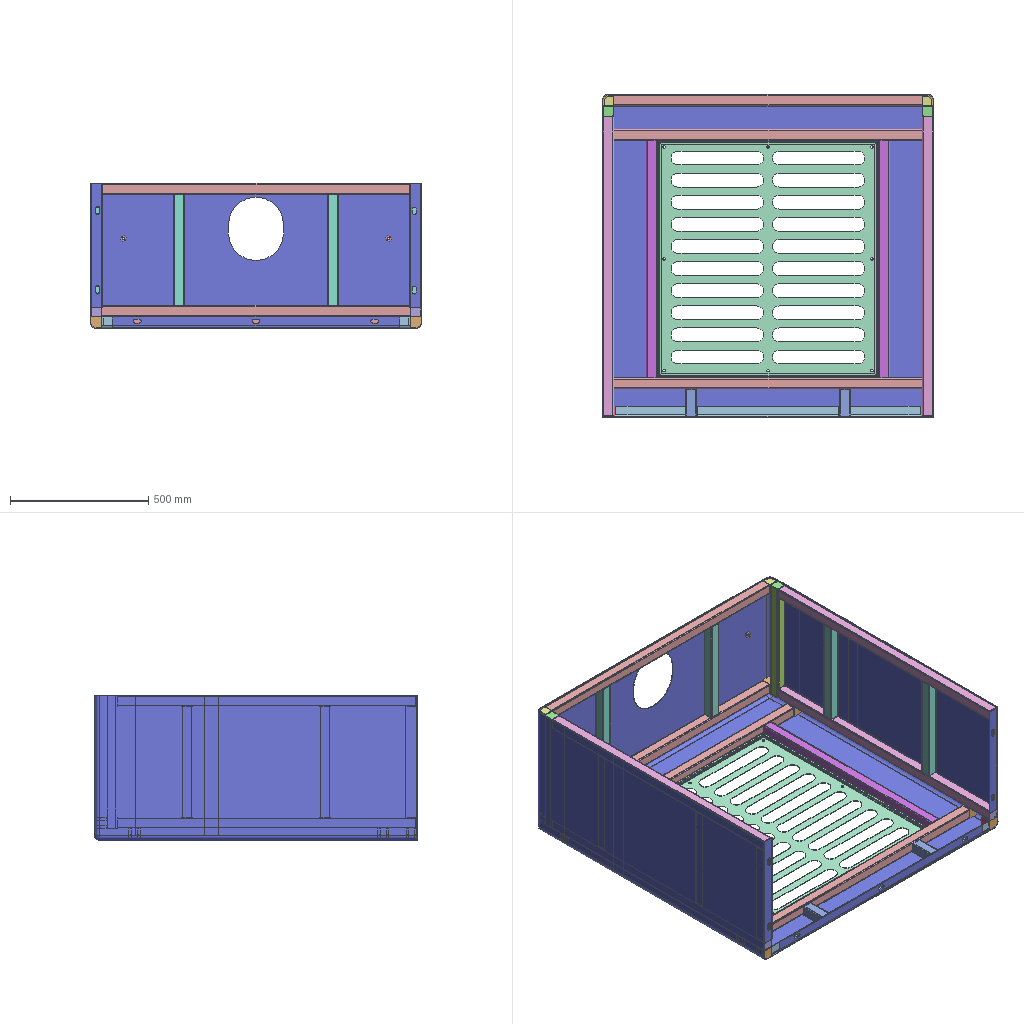Assembly | SolidWorks | 17 different items | 54 placed | box 1200 x 1170 x 527 mm
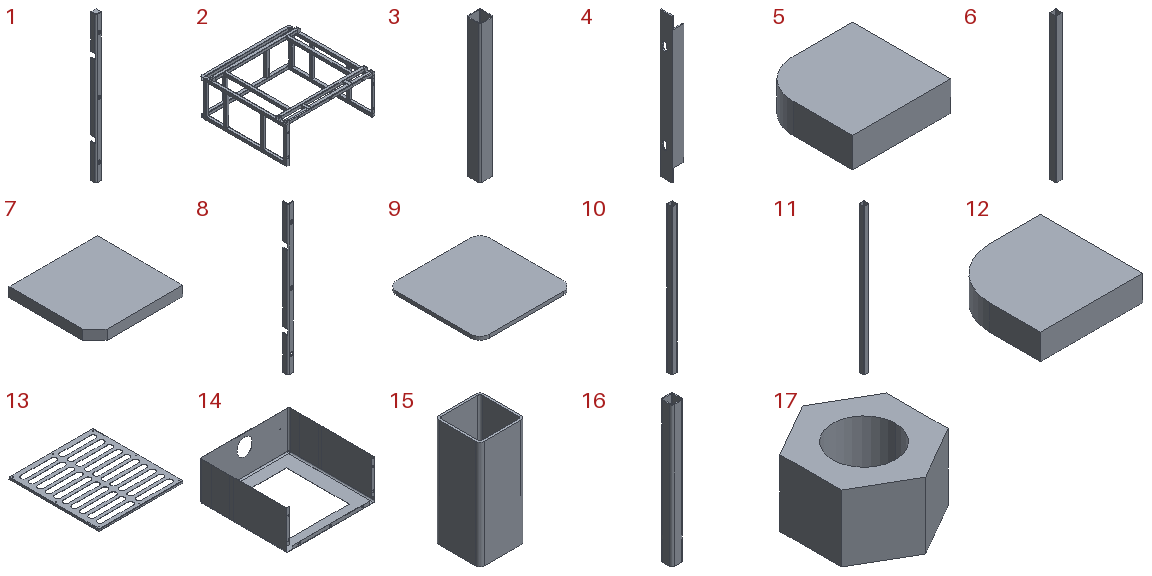Parts list (item | name | quantity | parent item | size | volume | features):
1 | (subassembly) | x1 | in 2 | 40 x 40 x 1116 mm | 321281 mm3 | -
2 | (subassembly) | x1 | - | 1196 x 1166 x 524.14 mm | 5123643 mm3 | features ReferencePattern 21, MirrorCompFeat 7, LocalLPattern 2
3 | - | x6 | in 2 | 40 x 40 x 403 mm | 118361 mm3 | features Fillet 2, Extrusion 1
4 | - | x2 | in 2 | 40 x 40 x 484.14 mm | 134390 mm3 | features ICE 3, Fillet 2, ExtruThin 1, LPattern 1
5 | - | x4 | in 2 | 33 x 33 x 10 mm | 10527 mm3 | features Extrusion 1, Fillet 1, ICE 1
6 | - | x2 | in 2 | 40 x 40 x 860 mm | 252581 mm3 | features Fillet 2, Extrusion 1
7 | - | x2 | in 1 | 36 x 35 x 4 mm | 4990 mm3 | features Chamfer 1, Extrusion 1
8 | - | x1 | in 1 | 40 x 40 x 1116 mm | 311301 mm3 | features ICE 2, LPattern 2, ExtruThin 1, RefAxis 1
9 | - | x3 | in 2 | 40 x 40 x 1.5 mm | 2379 mm3 | features Extrusion 1
10 | - | x4 | in 2 | 40 x 40 x 1082 mm | 317782 mm3 | features Fillet 2, Extrusion 1
11 | - | x4 | in 2 | 40 x 40 x 1116 mm | 327768 mm3 | features Fillet 2, Extrusion 1
12 | - | x16 | in 2 | 40 x 40 x 10 mm | 15142 mm3 | features Extrusion 1, Fillet 1
13 | - | x1 | - | 792 x 850 x 20 mm | 853821 mm3 | features ICE 3, EdgeFlange 2, LPattern 2, MirrorPattern 2, FlatPattern 1, SMBaseFlange 1, SheetMetal 1
14 | - | x1 | - | 1200 x 1170 x 527 mm | 5175590 mm3 | features ICE 9, Fillet 4, LPattern 3, MirrorPattern 3, Extrusion 1, Shell 1
15 | - | x2 | in 2 | 40 x 40 x 95 mm | 27901 mm3 | features Fillet 2, Extrusion 1
16 | - | x2 | in 2 | 40 x 40 x 479.48 mm | 194368 mm3 | features Fillet 2, Extrusion 1
17 | - | x2 | - | 17.3 x 19.976 x 10.8 mm | 1917 mm3 | features Extrusion 1, HoleWzd 1, RefAxis 1
Mates (type | each side: item.copy, entity, surface, feature):
In the top assembly
Coincident | 11.1 face plane Boss-Extrude1 | assembly plane
Coincident | 9.1 face plane Boss-Extrude1 | 14.1 face plane Boss-Extrude1
Coincident | 10.1 face plane Boss-Extrude1 | 14.1 face plane Shell1
Coincident | 4.1 face plane Extrude-Thin1 | 14.1 face plane Mirror1
Coincident | 13.1 face plane Base-Flange1 | 14.1 face plane Boss-Extrude1
Width | 13.1 face plane Edge-Flange1 | 13.1 face plane Edge-Flange1 | 14.1 face plane Cut-Extrude4 | 14.1 face plane Cut-Extrude4 | 2 times
Concentric | 17.1 face cylinder M12 Tapped Hole1 | 14.1 face cylinder Cut-Extrude5
Coincident | 17.1 face plane Boss-Extrude1 | 14.1 face plane Shell1
Concentric | 17.2 face cylinder M12 Tapped Hole1 | 14.1 face cylinder Mirror3
In subassembly 2
Coincident | 16.1 face plane Boss-Extrude1 | 10.2 face plane Boss-Extrude1 | 2 times
Coincident | 11.2 face plane Boss-Extrude1 | 12.1 face plane Boss-Extrude1 | 3 times
Coincident | 16.1 face plane Boss-Extrude1 | 12.1 face plane Boss-Extrude1 | 2 times
Coincident | 10.2 face plane Boss-Extrude1 | 4.2 face plane Extrude-Thin1 | 3 times
Coincident | 11.3 face plane Boss-Extrude1 | 12.2 face plane Boss-Extrude1 | 3 times
Coincident | 16.1 face plane Boss-Extrude1 | 9.2 face plane Boss-Extrude1 | 3 times
Coincident | 12.1 face plane Boss-Extrude1 | 9.2 face plane Boss-Extrude1
Coincident | 4.2 face plane Extrude-Thin1 | 8.1 face plane Extrude-Thin1
Coincident | 12.3 face plane Boss-Extrude1 | 7.1 face plane Boss-Extrude1
Coincident | 12.3 face plane Boss-Extrude1 | 8.1 face plane Extrude-Thin1
Coincident | 12.3 face plane Boss-Extrude1 | 7.1 vertex
Coincident | 11.2 face plane Boss-Extrude1 | 11.4 face plane Boss-Extrude1
Coincident | 16.1 face plane Boss-Extrude1 | 11.4 face plane Boss-Extrude1
Coincident | 10.2 face plane Boss-Extrude1 | 11.4 face plane Boss-Extrude1
Coincident | 16.1 face plane Boss-Extrude1 | 9.3 face plane Boss-Extrude1 | 3 times
Coincident | 3.1 face plane Boss-Extrude1 | 11.4 face plane Boss-Extrude1
Coincident | 11.2 face plane Boss-Extrude1 | 3.1 face plane Boss-Extrude1
DistanceDim | 11.3 edge | 8.1 face plane Extrude-Thin1
DistanceDim | 3.1 face plane Boss-Extrude1 | 16.1 face plane Boss-Extrude1
Coincident | 11.3 face plane Boss-Extrude1 | 15.1 face plane Boss-Extrude1
Coincident | 15.1 edge | 8.1 face plane Extrude-Thin1
Coincident | 11.2 face plane Boss-Extrude1 | 12.4 face plane Boss-Extrude1 | 2 times
Coincident | 16.1 face plane Boss-Extrude1 | 12.4 face plane Boss-Extrude1
Coincident | 12.2 face plane Boss-Extrude1 | 12.5 face plane Boss-Extrude1
Coincident | 11.3 face plane Boss-Extrude1 | 12.5 face plane Boss-Extrude1
Coincident | 11.4 face plane Boss-Extrude1 | 2.1 plane
Symmetric | 11.4 face plane Boss-Extrude1 | 11.4 face plane Boss-Extrude1 | 2.1 plane
Coincident | 4.2 face plane Extrude-Thin1 | 2.1 plane
Coincident | 10.2 face plane Boss-Extrude1 | 3.2 face plane Boss-Extrude1 | 2 times
Coincident | 11.4 face plane Boss-Extrude1 | 5.1 face plane Boss-Extrude1
Coincident | 16.1 face plane Boss-Extrude1 | 5.1 face plane Boss-Extrude1 | 2 times
Coincident | 16.1 face plane Boss-Extrude1 | 5.2 face plane Boss-Extrude1
Coincident | 11.4 face plane Boss-Extrude1 | 5.2 face plane Boss-Extrude1 | 2 times
Coincident | 15.1 face plane Boss-Extrude1 | 8.1 face plane Extrude-Thin1 | 2 times
Coincident | 4.2 face plane Extrude-Thin1 | 10.3 face plane Boss-Extrude1 | 2 times
Coincident | 4.3 face plane Extrude-Thin1 | 10.4 face plane Boss-Extrude1 | 3 times
Coincident | 11.3 face plane Boss-Extrude1 | 12.6 face plane Boss-Extrude1
Coincident | 12.7 face plane Boss-Extrude1 | 10.4 face plane Boss-Extrude1
Coincident | 11.3 face plane Boss-Extrude1 | 12.7 face plane Boss-Extrude1
Coincident | 4.2 face plane Cut-Extrude1 | 10.3 face plane Boss-Extrude1
Coincident | 15.1 face plane Boss-Extrude1 | 8.1 face plane Cut-Extrude1
Coincident | 10.2 face plane Boss-Extrude1 | 9.3 face plane Boss-Extrude1
Coincident | 12.3 face plane Boss-Extrude1 | 10.3 face plane Boss-Extrude1
Coincident | 12.3 edge | 12.8 face plane Boss-Extrude1
Coincident | 10.3 face plane Boss-Extrude1 | 12.8 face plane Boss-Extrude1
Coincident | 4.2 face plane Extrude-Thin1 | 12.8 face plane Boss-Extrude1
Coincident | 8.1 face plane Extrude-Thin1 | 12.9 face plane Boss-Extrude1 | 2 times
Coincident | 12.10 face plane Boss-Extrude1 | 12.9 face plane Boss-Extrude1
DistanceDim | 3.2 face plane Boss-Extrude1 | 4.2 face plane Extrude-Thin1
DistanceDim | 6.1 face plane Boss-Extrude1 | 6.2 face plane Boss-Extrude1
Coincident | 6.1 face plane Boss-Extrude1 | 6.2 face plane Boss-Extrude1 | 2 times
Coincident | 11.5 face plane Boss-Extrude1 | 6.1 face plane Boss-Extrude1
Coincident | 11.3 face plane Boss-Extrude1 | 6.2 face plane Boss-Extrude1
Width | 10.4 face plane Boss-Extrude1 | 10.3 face plane Boss-Extrude1 | 6.2 face plane Boss-Extrude1 | 6.1 face plane Boss-Extrude1
In subassembly 1
Coincident | 7.2 face plane Boss-Extrude1 | 8.2 face plane Extrude-Thin1 | 3 times
Coincident | 8.2 face plane Extrude-Thin1 | 7.3 face plane Boss-Extrude1
Coincident | 7.2 face plane Boss-Extrude1 | 7.3 face plane Boss-Extrude1 | 2 times